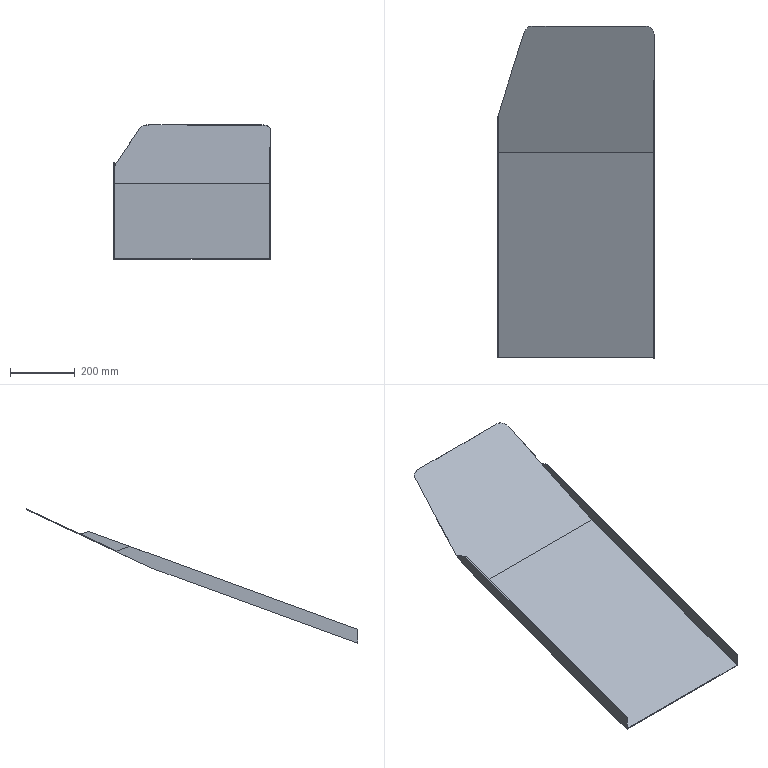Part | NX | features solid 2 | 1 solid | 17 faces | box 480.993 x 1021 x 413.434 mm | volume 1152601 mm3 | plane 14 | spline 3
STEP:
#1=CARTESIAN_POINT('',(108.81,-820.,-518.767));
#2=VERTEX_POINT('',#1);
#3=CARTESIAN_POINT('',(589.803,-820.,-518.767));
#4=VERTEX_POINT('',#3);
#5=CARTESIAN_POINT('',(1065.,-820.,-518.767));
#6=DIRECTION('',(-1.,0.,0.));
#7=VECTOR('',#6,1000.);
#8=LINE('',#5,#7);
#9=EDGE_CURVE('',#2,#4,#8,.F.);
#10=ORIENTED_EDGE('',*,*,#9,.T.);
#11=CARTESIAN_POINT('',(589.803,-820.,-476.2));
#12=VERTEX_POINT('',#11);
#13=CARTESIAN_POINT('',(589.803,-820.,-700.));
#14=DIRECTION('',(0.,0.,-1.));
#15=VECTOR('',#14,1000.);
#16=LINE('',#13,#15);
#17=EDGE_CURVE('',#12,#4,#16,.T.);
#18=ORIENTED_EDGE('',*,*,#17,.F.);
#19=CARTESIAN_POINT('',(587.803,-820.,-476.2));
#20=VERTEX_POINT('',#19);
#21=CARTESIAN_POINT('',(589.803,-820.,-476.2));
#22=DIRECTION('',(1.,0.,0.));
#23=VECTOR('',#22,1000.);
#24=LINE('',#21,#23);
#25=EDGE_CURVE('',#20,#12,#24,.T.);
#26=ORIENTED_EDGE('',*,*,#25,.F.);
#27=CARTESIAN_POINT('',(587.803,-820.,-516.639));
#28=VERTEX_POINT('',#27);
#29=CARTESIAN_POINT('',(587.803,-820.,-700.));
#30=DIRECTION('',(0.,0.,-1.));
#31=VECTOR('',#30,1000.);
#32=LINE('',#29,#31);
#33=EDGE_CURVE('',#28,#20,#32,.F.);
#34=ORIENTED_EDGE('',*,*,#33,.F.);
#35=CARTESIAN_POINT('',(110.81,-820.,-516.639));
#36=VERTEX_POINT('',#35);
#37=CARTESIAN_POINT('',(274.102,-820.,-516.639));
#38=DIRECTION('',(1.,0.,0.));
#39=VECTOR('',#38,1000.);
#40=LINE('',#37,#39);
#41=EDGE_CURVE('',#36,#28,#40,.T.);
#42=ORIENTED_EDGE('',*,*,#41,.F.);
#43=CARTESIAN_POINT('',(110.81,-820.,-476.2));
#44=VERTEX_POINT('',#43);
#45=CARTESIAN_POINT('',(110.81,-820.,-700.));
#46=DIRECTION('',(0.,0.,1.));
#47=VECTOR('',#46,1000.);
#48=LINE('',#45,#47);
#49=EDGE_CURVE('',#44,#36,#48,.F.);
#50=ORIENTED_EDGE('',*,*,#49,.F.);
#51=CARTESIAN_POINT('',(108.81,-820.,-476.2));
#52=VERTEX_POINT('',#51);
#53=CARTESIAN_POINT('',(1065.,-820.,-476.2));
#54=DIRECTION('',(1.,0.,0.));
#55=VECTOR('',#54,1000.);
#56=LINE('',#53,#55);
#57=EDGE_CURVE('',#52,#44,#56,.T.);
#58=ORIENTED_EDGE('',*,*,#57,.F.);
#59=CARTESIAN_POINT('',(108.81,-820.,-113.668));
#60=DIRECTION('',(0.,0.,1.));
#61=VECTOR('',#60,1000.);
#62=LINE('',#59,#61);
#63=EDGE_CURVE('',#2,#52,#62,.T.);
#64=ORIENTED_EDGE('',*,*,#63,.F.);
#65=EDGE_LOOP('',(#10,#18,#26,#34,#42,#50,#58,#64));
#66=FACE_BOUND('',#65,.T.);
#67=CARTESIAN_POINT('',(1065.,-820.,-700.));
#68=DIRECTION('',(0.,1.,0.));
#69=DIRECTION('',(-1.,0.,0.));
#70=AXIS2_PLACEMENT_3D('',#67,#68,#69);
#71=PLANE('',#70);
#72=ADVANCED_FACE('',(#66),#71,.F.);
#73=CARTESIAN_POINT('',(587.803,-186.962,-286.232));
#74=VERTEX_POINT('',#73);
#75=CARTESIAN_POINT('',(587.803,-188.342,-286.734));
#76=DIRECTION('',(0.,-0.9397,-0.342));
#77=VECTOR('',#76,1000.);
#78=LINE('',#75,#77);
#79=EDGE_CURVE('',#74,#28,#78,.T.);
#80=ORIENTED_EDGE('',*,*,#79,.F.);
#81=CARTESIAN_POINT('',(110.81,-186.962,-286.232));
#82=VERTEX_POINT('',#81);
#83=CARTESIAN_POINT('',(555.,-186.962,-286.232));
#84=DIRECTION('',(1.,0.,0.));
#85=VECTOR('',#84,1000.);
#86=LINE('',#83,#85);
#87=EDGE_CURVE('',#82,#74,#86,.T.);
#88=ORIENTED_EDGE('',*,*,#87,.F.);
#89=CARTESIAN_POINT('',(110.81,-188.342,-286.734));
#90=DIRECTION('',(0.,0.9397,0.342));
#91=VECTOR('',#90,1000.);
#92=LINE('',#89,#91);
#93=EDGE_CURVE('',#36,#82,#92,.T.);
#94=ORIENTED_EDGE('',*,*,#93,.F.);
#95=ORIENTED_EDGE('',*,*,#41,.T.);
#96=EDGE_LOOP('',(#80,#88,#94,#95));
#97=FACE_BOUND('',#96,.T.);
#98=CARTESIAN_POINT('',(274.102,-188.342,-286.734));
#99=DIRECTION('',(0.,0.342,-0.9397));
#100=DIRECTION('',(-1.,0.,0.));
#101=AXIS2_PLACEMENT_3D('',#98,#99,#100);
#102=PLANE('',#101);
#103=ADVANCED_FACE('',(#97),#102,.F.);
#104=ORIENTED_EDGE('',*,*,#87,.T.);
#105=CARTESIAN_POINT('',(587.803,32.739,-183.784));
#106=VERTEX_POINT('',#105);
#107=CARTESIAN_POINT('',(587.803,183.102,-113.668));
#108=DIRECTION('',(0.,0.9063,0.4226));
#109=VECTOR('',#108,1000.);
#110=LINE('',#107,#109);
#111=EDGE_CURVE('',#74,#106,#110,.T.);
#112=ORIENTED_EDGE('',*,*,#111,.T.);
#113=CARTESIAN_POINT('',(589.803,32.739,-183.784));
#114=VERTEX_POINT('',#113);
#115=CARTESIAN_POINT('',(589.803,32.739,-183.784));
#116=DIRECTION('',(1.,0.,0.));
#117=VECTOR('',#116,1000.);
#118=LINE('',#115,#117);
#119=EDGE_CURVE('',#106,#114,#118,.T.);
#120=ORIENTED_EDGE('',*,*,#119,.T.);
#121=CARTESIAN_POINT('',(589.803,33.584,-183.39));
#122=VERTEX_POINT('',#121);
#123=CARTESIAN_POINT('',(589.803,183.102,-113.668));
#124=DIRECTION('',(0.,-0.9063,-0.4226));
#125=VECTOR('',#124,1000.);
#126=LINE('',#123,#125);
#127=EDGE_CURVE('',#122,#114,#126,.T.);
#128=ORIENTED_EDGE('',*,*,#127,.F.);
#129=CARTESIAN_POINT('',(589.803,144.66,-131.594));
#130=VERTEX_POINT('',#129);
#131=CARTESIAN_POINT('',(589.803,33.584,-183.39));
#132=CARTESIAN_POINT('',(589.803,70.609,-166.125));
#133=CARTESIAN_POINT('',(589.803,107.634,-148.859));
#134=CARTESIAN_POINT('',(589.803,144.66,-131.594));
#135=B_SPLINE_CURVE_WITH_KNOTS('',3,(#131,#132,#133,#134),.UNSPECIFIED.,.F.,.F.,(4,4),(0.,1.),.UNSPECIFIED.);
#136=EDGE_CURVE('',#130,#122,#135,.F.);
#137=ORIENTED_EDGE('',*,*,#136,.F.);
#138=CARTESIAN_POINT('',(589.803,176.289,-116.845));
#139=VERTEX_POINT('',#138);
#140=CARTESIAN_POINT('',(589.803,183.102,-113.668));
#141=DIRECTION('',(0.,-0.9063,-0.4226));
#142=VECTOR('',#141,1000.);
#143=LINE('',#140,#142);
#144=EDGE_CURVE('',#139,#130,#143,.T.);
#145=ORIENTED_EDGE('',*,*,#144,.F.);
#146=CARTESIAN_POINT('',(374.989,200.501,-105.555));
#147=VERTEX_POINT('',#146);
#148=CARTESIAN_POINT('',(589.803,176.289,-116.845));
#149=CARTESIAN_POINT('',(589.689,178.459,-115.833));
#150=CARTESIAN_POINT('',(589.039,182.718,-113.847));
#151=CARTESIAN_POINT('',(586.3,188.791,-111.016));
#152=CARTESIAN_POINT('',(582.012,194.011,-108.581));
#153=CARTESIAN_POINT('',(576.33,198.,-106.721));
#154=CARTESIAN_POINT('',(569.521,200.317,-105.641));
#155=CARTESIAN_POINT('',(562.281,200.46,-105.574));
#156=CARTESIAN_POINT('',(555.087,200.407,-105.599));
#157=CARTESIAN_POINT('',(547.881,200.41,-105.597));
#158=CARTESIAN_POINT('',(540.677,200.401,-105.601));
#159=CARTESIAN_POINT('',(531.072,200.398,-105.603));
#160=CARTESIAN_POINT('',(519.066,200.397,-105.604));
#161=CARTESIAN_POINT('',(504.658,200.401,-105.602));
#162=CARTESIAN_POINT('',(485.448,200.411,-105.597));
#163=CARTESIAN_POINT('',(461.435,200.427,-105.59));
#164=CARTESIAN_POINT('',(432.62,200.445,-105.581));
#165=CARTESIAN_POINT('',(403.804,200.47,-105.569));
#166=CARTESIAN_POINT('',(384.594,200.49,-105.56));
#167=CARTESIAN_POINT('',(374.989,200.501,-105.555));
#168=B_SPLINE_CURVE_WITH_KNOTS('',3,(#148,#149,#150,#151,#152,#153,#154,#155,#156,#157,#158,#159,#160,#161,#162,#163,#164,#165,#166,#167),.UNSPECIFIED.,.F.,.F.,(4,1,1,1,1,1,1,1,1,1,1,1,1,1,1,1,1,4),(0.,0.007104,0.01421,0.02131,0.02842,0.03552,0.04263,0.04973,0.05683,0.06394,0.07104,0.08525,0.09946,0.1137,0.1421,0.1705,0.1989,0.2273),.UNSPECIFIED.);
#169=EDGE_CURVE('',#139,#147,#168,.T.);
#170=ORIENTED_EDGE('',*,*,#169,.T.);
#171=CARTESIAN_POINT('',(108.81,-77.408,-235.146));
#172=VERTEX_POINT('',#171);
#173=CARTESIAN_POINT('',(374.989,200.501,-105.555));
#174=CARTESIAN_POINT('',(364.858,200.512,-105.55));
#175=CARTESIAN_POINT('',(344.595,200.537,-105.538));
#176=CARTESIAN_POINT('',(319.267,200.578,-105.519));
#177=CARTESIAN_POINT('',(299.005,200.618,-105.5));
#178=CARTESIAN_POINT('',(283.808,200.655,-105.483));
#179=CARTESIAN_POINT('',(268.611,200.701,-105.462));
#180=CARTESIAN_POINT('',(253.415,200.754,-105.437));
#181=CARTESIAN_POINT('',(240.751,200.83,-105.402));
#182=CARTESIAN_POINT('',(230.62,200.892,-105.372));
#183=CARTESIAN_POINT('',(223.022,200.942,-105.349));
#184=CARTESIAN_POINT('',(216.683,201.04,-105.304));
#185=CARTESIAN_POINT('',(211.664,200.417,-105.594));
#186=CARTESIAN_POINT('',(206.634,199.19,-106.166));
#187=CARTESIAN_POINT('',(200.857,196.591,-107.378));
#188=CARTESIAN_POINT('',(195.037,191.859,-109.585));
#189=CARTESIAN_POINT('',(190.69,185.963,-112.334));
#190=CARTESIAN_POINT('',(187.958,179.442,-115.375));
#191=CARTESIAN_POINT('',(185.967,172.644,-118.545));
#192=CARTESIAN_POINT('',(183.9,165.886,-121.696));
#193=CARTESIAN_POINT('',(181.808,159.128,-124.848));
#194=CARTESIAN_POINT('',(179.029,150.117,-129.049));
#195=CARTESIAN_POINT('',(175.562,138.851,-134.303));
#196=CARTESIAN_POINT('',(171.409,125.33,-140.608));
#197=CARTESIAN_POINT('',(165.867,107.303,-149.014));
#198=CARTESIAN_POINT('',(158.92,84.774,-159.519));
#199=CARTESIAN_POINT('',(150.571,57.743,-172.124));
#200=CARTESIAN_POINT('',(142.222,30.712,-184.729));
#201=CARTESIAN_POINT('',(133.888,3.677,-197.335));
#202=CARTESIAN_POINT('',(122.783,-32.371,-214.145));
#203=CARTESIAN_POINT('',(114.391,-59.391,-226.745));
#204=CARTESIAN_POINT('',(108.81,-77.408,-235.146));
#205=B_SPLINE_CURVE_WITH_KNOTS('',3,(#173,#174,#175,#176,#177,#178,#179,#180,#181,#182,#183,#184,#185,#186,#187,#188,#189,#190,#191,#192,#193,#194,#195,#196,#197,#198,#199,#200,#201,#202,#203,#204),.UNSPECIFIED.,.F.,.F.,(4,1,1,1,1,1,1,1,1,1,1,1,1,1,1,1,1,1,1,1,1,1,1,1,1,1,1,1,1,4),(0.,0.03039,0.06079,0.07598,0.09118,0.1064,0.1216,0.1368,0.1444,0.152,0.1596,0.1634,0.1672,0.1748,0.1824,0.19,0.1976,0.2052,0.2128,0.2204,0.228,0.2431,0.2583,0.2735,0.3039,0.3343,0.3647,0.3951,0.4255,0.4863),.UNSPECIFIED.);
#206=EDGE_CURVE('',#147,#172,#205,.T.);
#207=ORIENTED_EDGE('',*,*,#206,.T.);
#208=CARTESIAN_POINT('',(108.81,-78.254,-235.54));
#209=VERTEX_POINT('',#208);
#210=CARTESIAN_POINT('',(108.81,183.102,-113.668));
#211=DIRECTION('',(0.,-0.9063,-0.4226));
#212=VECTOR('',#211,1000.);
#213=LINE('',#210,#212);
#214=EDGE_CURVE('',#172,#209,#213,.T.);
#215=ORIENTED_EDGE('',*,*,#214,.T.);
#216=CARTESIAN_POINT('',(110.81,-78.254,-235.54));
#217=VERTEX_POINT('',#216);
#218=CARTESIAN_POINT('',(110.81,-78.254,-235.54));
#219=DIRECTION('',(1.,0.,0.));
#220=VECTOR('',#219,1000.);
#221=LINE('',#218,#220);
#222=EDGE_CURVE('',#209,#217,#221,.T.);
#223=ORIENTED_EDGE('',*,*,#222,.T.);
#224=CARTESIAN_POINT('',(110.81,183.102,-113.668));
#225=DIRECTION('',(0.,-0.9063,-0.4226));
#226=VECTOR('',#225,1000.);
#227=LINE('',#224,#226);
#228=EDGE_CURVE('',#217,#82,#227,.T.);
#229=ORIENTED_EDGE('',*,*,#228,.T.);
#230=EDGE_LOOP('',(#104,#112,#120,#128,#137,#145,#170,#207,#215,#223,#229));
#231=FACE_BOUND('',#230,.T.);
#232=CARTESIAN_POINT('',(555.,183.102,-113.668));
#233=DIRECTION('',(0.,-0.4226,0.9063));
#234=DIRECTION('',(1.,0.,0.));
#235=AXIS2_PLACEMENT_3D('',#232,#233,#234);
#236=PLANE('',#235);
#237=ADVANCED_FACE('',(#231),#236,.T.);
#238=CARTESIAN_POINT('',(589.803,144.66,-133.801));
#239=VERTEX_POINT('',#238);
#240=CARTESIAN_POINT('',(589.803,33.584,-185.596));
#241=VERTEX_POINT('',#240);
#242=CARTESIAN_POINT('',(589.803,144.66,-133.801));
#243=CARTESIAN_POINT('',(589.803,107.634,-151.066));
#244=CARTESIAN_POINT('',(589.803,70.609,-168.331));
#245=CARTESIAN_POINT('',(589.803,33.584,-185.596));
#246=B_SPLINE_CURVE_WITH_KNOTS('',3,(#242,#243,#244,#245),.UNSPECIFIED.,.F.,.F.,(4,4),(0.,1.),.UNSPECIFIED.);
#247=EDGE_CURVE('',#239,#241,#246,.T.);
#248=ORIENTED_EDGE('',*,*,#247,.T.);
#249=CARTESIAN_POINT('',(589.803,-186.196,-288.081));
#250=VERTEX_POINT('',#249);
#251=CARTESIAN_POINT('',(589.803,183.947,-115.481));
#252=DIRECTION('',(0.,-0.9063,-0.4226));
#253=VECTOR('',#252,1000.);
#254=LINE('',#251,#253);
#255=EDGE_CURVE('',#250,#241,#254,.F.);
#256=ORIENTED_EDGE('',*,*,#255,.F.);
#257=CARTESIAN_POINT('',(108.81,-186.196,-288.081));
#258=VERTEX_POINT('',#257);
#259=CARTESIAN_POINT('',(274.102,-186.196,-288.081));
#260=DIRECTION('',(-1.,0.,0.));
#261=VECTOR('',#260,1000.);
#262=LINE('',#259,#261);
#263=EDGE_CURVE('',#258,#250,#262,.F.);
#264=ORIENTED_EDGE('',*,*,#263,.F.);
#265=CARTESIAN_POINT('',(108.81,-77.408,-237.353));
#266=VERTEX_POINT('',#265);
#267=CARTESIAN_POINT('',(108.81,183.947,-115.481));
#268=DIRECTION('',(0.,-0.9063,-0.4226));
#269=VECTOR('',#268,1000.);
#270=LINE('',#267,#269);
#271=EDGE_CURVE('',#258,#266,#270,.F.);
#272=ORIENTED_EDGE('',*,*,#271,.T.);
#273=CARTESIAN_POINT('',(374.989,200.501,-107.762));
#274=VERTEX_POINT('',#273);
#275=CARTESIAN_POINT('',(374.989,200.501,-107.762));
#276=CARTESIAN_POINT('',(364.858,200.512,-107.756));
#277=CARTESIAN_POINT('',(344.595,200.537,-107.745));
#278=CARTESIAN_POINT('',(319.267,200.578,-107.726));
#279=CARTESIAN_POINT('',(299.005,200.618,-107.707));
#280=CARTESIAN_POINT('',(283.808,200.655,-107.69));
#281=CARTESIAN_POINT('',(268.611,200.701,-107.669));
#282=CARTESIAN_POINT('',(253.415,200.754,-107.644));
#283=CARTESIAN_POINT('',(240.751,200.83,-107.608));
#284=CARTESIAN_POINT('',(230.62,200.892,-107.579));
#285=CARTESIAN_POINT('',(223.022,200.942,-107.556));
#286=CARTESIAN_POINT('',(216.683,201.04,-107.51));
#287=CARTESIAN_POINT('',(211.664,200.417,-107.801));
#288=CARTESIAN_POINT('',(206.634,199.19,-108.373));
#289=CARTESIAN_POINT('',(200.857,196.591,-109.585));
#290=CARTESIAN_POINT('',(195.037,191.859,-111.792));
#291=CARTESIAN_POINT('',(190.69,185.963,-114.541));
#292=CARTESIAN_POINT('',(187.958,179.442,-117.582));
#293=CARTESIAN_POINT('',(185.967,172.644,-120.752));
#294=CARTESIAN_POINT('',(183.9,165.886,-123.903));
#295=CARTESIAN_POINT('',(181.808,159.128,-127.054));
#296=CARTESIAN_POINT('',(179.029,150.117,-131.256));
#297=CARTESIAN_POINT('',(175.562,138.851,-136.51));
#298=CARTESIAN_POINT('',(171.409,125.33,-142.815));
#299=CARTESIAN_POINT('',(165.867,107.303,-151.221));
#300=CARTESIAN_POINT('',(158.92,84.774,-161.726));
#301=CARTESIAN_POINT('',(150.571,57.743,-174.331));
#302=CARTESIAN_POINT('',(142.222,30.712,-186.936));
#303=CARTESIAN_POINT('',(133.888,3.677,-199.542));
#304=CARTESIAN_POINT('',(122.783,-32.371,-216.352));
#305=CARTESIAN_POINT('',(114.391,-59.391,-228.951));
#306=CARTESIAN_POINT('',(108.81,-77.408,-237.353));
#307=B_SPLINE_CURVE_WITH_KNOTS('',3,(#275,#276,#277,#278,#279,#280,#281,#282,#283,#284,#285,#286,#287,#288,#289,#290,#291,#292,#293,#294,#295,#296,#297,#298,#299,#300,#301,#302,#303,#304,#305,#306),.UNSPECIFIED.,.F.,.F.,(4,1,1,1,1,1,1,1,1,1,1,1,1,1,1,1,1,1,1,1,1,1,1,1,1,1,1,1,1,4),(0.,0.03039,0.06079,0.07598,0.09118,0.1064,0.1216,0.1368,0.1444,0.152,0.1596,0.1634,0.1672,0.1748,0.1824,0.19,0.1976,0.2052,0.2128,0.2204,0.228,0.2431,0.2583,0.2735,0.3039,0.3343,0.3647,0.3951,0.4255,0.4863),.UNSPECIFIED.);
#308=EDGE_CURVE('',#274,#266,#307,.T.);
#309=ORIENTED_EDGE('',*,*,#308,.F.);
#310=CARTESIAN_POINT('',(589.803,176.289,-119.052));
#311=VERTEX_POINT('',#310);
#312=CARTESIAN_POINT('',(589.803,176.289,-119.052));
#313=CARTESIAN_POINT('',(589.689,178.459,-118.04));
#314=CARTESIAN_POINT('',(589.039,182.718,-116.054));
#315=CARTESIAN_POINT('',(586.3,188.791,-113.222));
#316=CARTESIAN_POINT('',(582.012,194.011,-110.788));
#317=CARTESIAN_POINT('',(576.33,198.,-108.928));
#318=CARTESIAN_POINT('',(569.521,200.317,-107.848));
#319=CARTESIAN_POINT('',(562.281,200.46,-107.781));
#320=CARTESIAN_POINT('',(555.087,200.407,-107.805));
#321=CARTESIAN_POINT('',(547.881,200.41,-107.804));
#322=CARTESIAN_POINT('',(540.677,200.401,-107.808));
#323=CARTESIAN_POINT('',(531.072,200.398,-107.81));
#324=CARTESIAN_POINT('',(519.066,200.397,-107.81));
#325=CARTESIAN_POINT('',(504.658,200.401,-107.808));
#326=CARTESIAN_POINT('',(485.448,200.411,-107.804));
#327=CARTESIAN_POINT('',(461.435,200.427,-107.796));
#328=CARTESIAN_POINT('',(432.62,200.445,-107.788));
#329=CARTESIAN_POINT('',(403.804,200.47,-107.776));
#330=CARTESIAN_POINT('',(384.594,200.49,-107.767));
#331=CARTESIAN_POINT('',(374.989,200.501,-107.762));
#332=B_SPLINE_CURVE_WITH_KNOTS('',3,(#312,#313,#314,#315,#316,#317,#318,#319,#320,#321,#322,#323,#324,#325,#326,#327,#328,#329,#330,#331),.UNSPECIFIED.,.F.,.F.,(4,1,1,1,1,1,1,1,1,1,1,1,1,1,1,1,1,4),(0.,0.007104,0.01421,0.02131,0.02842,0.03552,0.04263,0.04973,0.05683,0.06394,0.07104,0.08525,0.09946,0.1137,0.1421,0.1705,0.1989,0.2273),.UNSPECIFIED.);
#333=EDGE_CURVE('',#311,#274,#332,.T.);
#334=ORIENTED_EDGE('',*,*,#333,.F.);
#335=CARTESIAN_POINT('',(589.803,183.947,-115.481));
#336=DIRECTION('',(0.,-0.9063,-0.4226));
#337=VECTOR('',#336,1000.);
#338=LINE('',#335,#337);
#339=EDGE_CURVE('',#311,#239,#338,.T.);
#340=ORIENTED_EDGE('',*,*,#339,.T.);
#341=EDGE_LOOP('',(#248,#256,#264,#272,#309,#334,#340));
#342=FACE_BOUND('',#341,.T.);
#343=CARTESIAN_POINT('',(555.,183.947,-115.481));
#344=DIRECTION('',(0.,-0.4226,0.9063));
#345=DIRECTION('',(1.,0.,0.));
#346=AXIS2_PLACEMENT_3D('',#343,#344,#345);
#347=PLANE('',#346);
#348=ADVANCED_FACE('',(#342),#347,.F.);
#349=CARTESIAN_POINT('',(589.803,-187.658,-288.613));
#350=DIRECTION('',(0.,-0.9397,-0.342));
#351=VECTOR('',#350,1000.);
#352=LINE('',#349,#351);
#353=EDGE_CURVE('',#250,#4,#352,.T.);
#354=ORIENTED_EDGE('',*,*,#353,.T.);
#355=ORIENTED_EDGE('',*,*,#9,.F.);
#356=CARTESIAN_POINT('',(108.81,-187.658,-288.613));
#357=DIRECTION('',(0.,-0.9397,-0.342));
#358=VECTOR('',#357,1000.);
#359=LINE('',#356,#358);
#360=EDGE_CURVE('',#258,#2,#359,.T.);
#361=ORIENTED_EDGE('',*,*,#360,.F.);
#362=ORIENTED_EDGE('',*,*,#263,.T.);
#363=EDGE_LOOP('',(#354,#355,#361,#362));
#364=FACE_BOUND('',#363,.T.);
#365=CARTESIAN_POINT('',(274.102,-187.658,-288.613));
#366=DIRECTION('',(0.,0.342,-0.9397));
#367=DIRECTION('',(-1.,0.,0.));
#368=AXIS2_PLACEMENT_3D('',#365,#366,#367);
#369=PLANE('',#368);
#370=ADVANCED_FACE('',(#364),#369,.T.);
#371=ORIENTED_EDGE('',*,*,#360,.T.);
#372=ORIENTED_EDGE('',*,*,#63,.T.);
#373=CARTESIAN_POINT('',(108.81,-118.523,-220.883));
#374=VERTEX_POINT('',#373);
#375=CARTESIAN_POINT('',(108.81,182.276,-111.401));
#376=DIRECTION('',(0.,-0.9397,-0.342));
#377=VECTOR('',#376,1000.);
#378=LINE('',#375,#377);
#379=EDGE_CURVE('',#374,#52,#378,.T.);
#380=ORIENTED_EDGE('',*,*,#379,.F.);
#381=CARTESIAN_POINT('',(108.81,-78.254,-235.54));
#382=DIRECTION('',(0.,-0.9397,0.342));
#383=VECTOR('',#382,1000.);
#384=LINE('',#381,#383);
#385=EDGE_CURVE('',#374,#209,#384,.F.);
#386=ORIENTED_EDGE('',*,*,#385,.T.);
#387=ORIENTED_EDGE('',*,*,#214,.F.);
#388=CARTESIAN_POINT('',(108.81,-77.408,-1000.));
#389=DIRECTION('',(0.,0.,1.));
#390=VECTOR('',#389,1000.);
#391=LINE('',#388,#390);
#392=EDGE_CURVE('',#266,#172,#391,.T.);
#393=ORIENTED_EDGE('',*,*,#392,.F.);
#394=ORIENTED_EDGE('',*,*,#271,.F.);
#395=EDGE_LOOP('',(#371,#372,#380,#386,#387,#393,#394));
#396=FACE_BOUND('',#395,.T.);
#397=CARTESIAN_POINT('',(108.81,183.102,-113.668));
#398=DIRECTION('',(1.,0.,0.));
#399=DIRECTION('',(0.,0.,-1.));
#400=AXIS2_PLACEMENT_3D('',#397,#398,#399);
#401=PLANE('',#400);
#402=ADVANCED_FACE('',(#396),#401,.F.);
#403=ORIENTED_EDGE('',*,*,#17,.T.);
#404=ORIENTED_EDGE('',*,*,#353,.F.);
#405=ORIENTED_EDGE('',*,*,#255,.T.);
#406=CARTESIAN_POINT('',(589.803,33.584,-1000.));
#407=DIRECTION('',(0.,0.,1.));
#408=VECTOR('',#407,1000.);
#409=LINE('',#406,#408);
#410=EDGE_CURVE('',#241,#122,#409,.T.);
#411=ORIENTED_EDGE('',*,*,#410,.T.);
#412=ORIENTED_EDGE('',*,*,#127,.T.);
#413=CARTESIAN_POINT('',(589.803,8.073,-174.806));
#414=VERTEX_POINT('',#413);
#415=CARTESIAN_POINT('',(589.803,8.818,-175.077));
#416=DIRECTION('',(0.,-0.9397,0.342));
#417=VECTOR('',#416,1000.);
#418=LINE('',#415,#417);
#419=EDGE_CURVE('',#114,#414,#418,.T.);
#420=ORIENTED_EDGE('',*,*,#419,.T.);
#421=CARTESIAN_POINT('',(589.803,-199.877,-250.494));
#422=DIRECTION('',(0.,-0.9397,-0.342));
#423=VECTOR('',#422,1000.);
#424=LINE('',#421,#423);
#425=EDGE_CURVE('',#414,#12,#424,.T.);
#426=ORIENTED_EDGE('',*,*,#425,.T.);
#427=EDGE_LOOP('',(#403,#404,#405,#411,#412,#420,#426));
#428=FACE_BOUND('',#427,.T.);
#429=CARTESIAN_POINT('',(589.803,183.102,-113.668));
#430=DIRECTION('',(1.,0.,0.));
#431=DIRECTION('',(0.,0.,-1.));
#432=AXIS2_PLACEMENT_3D('',#429,#430,#431);
#433=PLANE('',#432);
#434=ADVANCED_FACE('',(#428),#433,.T.);
#435=ORIENTED_EDGE('',*,*,#206,.F.);
#436=CARTESIAN_POINT('',(374.989,200.501,-1000.));
#437=DIRECTION('',(0.,0.,1.));
#438=VECTOR('',#437,1000.);
#439=LINE('',#436,#438);
#440=EDGE_CURVE('',#274,#147,#439,.T.);
#441=ORIENTED_EDGE('',*,*,#440,.F.);
#442=ORIENTED_EDGE('',*,*,#308,.T.);
#443=ORIENTED_EDGE('',*,*,#392,.T.);
#444=EDGE_LOOP('',(#435,#441,#442,#443));
#445=FACE_BOUND('',#444,.T.);
#446=CARTESIAN_POINT('',(374.989,200.501,-238.148));
#447=CARTESIAN_POINT('',(374.989,200.501,-104.13));
#448=CARTESIAN_POINT('',(365.187,200.512,-238.148));
#449=CARTESIAN_POINT('',(365.187,200.512,-104.13));
#450=CARTESIAN_POINT('',(345.583,200.536,-238.148));
#451=CARTESIAN_POINT('',(345.583,200.536,-104.13));
#452=CARTESIAN_POINT('',(316.178,200.583,-238.148));
#453=CARTESIAN_POINT('',(316.178,200.583,-104.13));
#454=CARTESIAN_POINT('',(291.673,200.633,-238.148));
#455=CARTESIAN_POINT('',(291.673,200.633,-104.13));
#456=CARTESIAN_POINT('',(272.069,200.689,-238.148));
#457=CARTESIAN_POINT('',(272.069,200.689,-104.13));
#458=CARTESIAN_POINT('',(257.367,200.742,-238.148));
#459=CARTESIAN_POINT('',(257.367,200.742,-104.13));
#460=CARTESIAN_POINT('',(245.114,200.793,-238.148));
#461=CARTESIAN_POINT('',(245.114,200.793,-104.13));
#462=CARTESIAN_POINT('',(235.313,200.874,-238.148));
#463=CARTESIAN_POINT('',(235.313,200.874,-104.13));
#464=CARTESIAN_POINT('',(227.961,200.88,-238.148));
#465=CARTESIAN_POINT('',(227.961,200.88,-104.13));
#466=CARTESIAN_POINT('',(220.611,201.039,-238.148));
#467=CARTESIAN_POINT('',(220.611,201.039,-104.13));
#468=CARTESIAN_POINT('',(213.256,200.864,-238.148));
#469=CARTESIAN_POINT('',(213.256,200.864,-104.13));
#470=CARTESIAN_POINT('',(206.093,199.101,-238.148));
#471=CARTESIAN_POINT('',(206.093,199.101,-104.13));
#472=CARTESIAN_POINT('',(199.581,195.744,-238.148));
#473=CARTESIAN_POINT('',(199.581,195.744,-104.13));
#474=CARTESIAN_POINT('',(194.084,190.795,-238.148));
#475=CARTESIAN_POINT('',(194.084,190.795,-104.13));
#476=CARTESIAN_POINT('',(189.965,184.643,-238.148));
#477=CARTESIAN_POINT('',(189.965,184.643,-104.13));
#478=CARTESIAN_POINT('',(187.476,177.842,-238.148));
#479=CARTESIAN_POINT('',(187.476,177.842,-104.13));
#480=CARTESIAN_POINT('',(185.452,170.916,-238.148));
#481=CARTESIAN_POINT('',(185.452,170.916,-104.13));
#482=CARTESIAN_POINT('',(183.32,164.017,-238.148));
#483=CARTESIAN_POINT('',(183.32,164.017,-104.13));
#484=CARTESIAN_POINT('',(180.478,154.822,-238.148));
#485=CARTESIAN_POINT('',(180.478,154.822,-104.13));
#486=CARTESIAN_POINT('',(176.937,143.323,-238.148));
#487=CARTESIAN_POINT('',(176.937,143.323,-104.13));
#488=CARTESIAN_POINT('',(172.697,129.522,-238.148));
#489=CARTESIAN_POINT('',(172.697,129.522,-104.13));
#490=CARTESIAN_POINT('',(167.043,111.12,-238.148));
#491=CARTESIAN_POINT('',(167.043,111.12,-104.13));
#492=CARTESIAN_POINT('',(159.955,88.125,-238.148));
#493=CARTESIAN_POINT('',(159.955,88.125,-104.13));
#494=CARTESIAN_POINT('',(151.434,60.535,-238.148));
#495=CARTESIAN_POINT('',(151.434,60.535,-104.13));
#496=CARTESIAN_POINT('',(142.911,32.946,-238.148));
#497=CARTESIAN_POINT('',(142.911,32.946,-104.13));
#498=CARTESIAN_POINT('',(134.404,5.352,-238.148));
#499=CARTESIAN_POINT('',(134.404,5.352,-104.13));
#500=CARTESIAN_POINT('',(123.07,-31.443,-238.148));
#501=CARTESIAN_POINT('',(123.07,-31.443,-104.13));
#502=CARTESIAN_POINT('',(114.506,-59.02,-238.148));
#503=CARTESIAN_POINT('',(114.506,-59.02,-104.13));
#504=CARTESIAN_POINT('',(108.81,-77.408,-238.148));
#505=CARTESIAN_POINT('',(108.81,-77.408,-104.13));
#506=B_SPLINE_SURFACE_WITH_KNOTS('',3,1,((#446,#447),(#448,#449),(#450,#451),(#452,#453),(#454,#455),(#456,#457),(#458,#459),(#460,#461),(#462,#463),(#464,#465),(#466,#467),(#468,#469),(#470,#471),(#472,#473),(#474,#475),(#476,#477),(#478,#479),(#480,#481),(#482,#483),(#484,#485),(#486,#487),(#488,#489),(#490,#491),(#492,#493),(#494,#495),(#496,#497),(#498,#499),(#500,#501),(#502,#503),(#504,#505)),.SURF_OF_LINEAR_EXTRUSION.,.F.,.F.,.F.,(4,1,1,1,1,1,1,1,1,1,1,1,1,1,1,1,1,1,1,1,1,1,1,1,1,1,1,4),(2,2),(0.,0.03647,0.07294,0.1094,0.1276,0.1459,0.1641,0.1732,0.1823,0.1915,0.2006,0.2097,0.2188,0.2279,0.237,0.2462,0.2553,0.2644,0.2735,0.2917,0.31,0.3282,0.3647,0.4011,0.4376,0.4741,0.5105,0.5835),(0.,1.),.UNSPECIFIED.);
#507=ADVANCED_FACE('',(#445),#506,.T.);
#508=ORIENTED_EDGE('',*,*,#169,.F.);
#509=CARTESIAN_POINT('',(589.803,176.289,-1000.));
#510=DIRECTION('',(0.,0.,1.));
#511=VECTOR('',#510,1000.);
#512=LINE('',#509,#511);
#513=EDGE_CURVE('',#311,#139,#512,.T.);
#514=ORIENTED_EDGE('',*,*,#513,.F.);
#515=ORIENTED_EDGE('',*,*,#333,.T.);
#516=ORIENTED_EDGE('',*,*,#440,.T.);
#517=EDGE_LOOP('',(#508,#514,#515,#516));
#518=FACE_BOUND('',#517,.T.);
#519=CARTESIAN_POINT('',(589.803,176.289,-119.135));
#520=CARTESIAN_POINT('',(589.803,176.289,-105.202));
#521=CARTESIAN_POINT('',(589.678,178.665,-119.135));
#522=CARTESIAN_POINT('',(589.678,178.665,-105.202));
#523=CARTESIAN_POINT('',(588.891,183.392,-119.135));
#524=CARTESIAN_POINT('',(588.891,183.392,-105.202));
#525=CARTESIAN_POINT('',(585.663,189.846,-119.135));
#526=CARTESIAN_POINT('',(585.663,189.846,-105.202));
#527=CARTESIAN_POINT('',(580.768,195.13,-119.135));
#528=CARTESIAN_POINT('',(580.768,195.13,-105.202));
#529=CARTESIAN_POINT('',(574.583,198.83,-119.135));
#530=CARTESIAN_POINT('',(574.583,198.83,-105.202));
#531=CARTESIAN_POINT('',(567.576,200.534,-119.135));
#532=CARTESIAN_POINT('',(567.576,200.534,-105.202));
#533=CARTESIAN_POINT('',(560.418,200.398,-119.135));
#534=CARTESIAN_POINT('',(560.418,200.398,-105.202));
#535=CARTESIAN_POINT('',(553.293,200.42,-119.135));
#536=CARTESIAN_POINT('',(553.293,200.42,-105.202));
#537=CARTESIAN_POINT('',(543.781,200.4,-119.135));
#538=CARTESIAN_POINT('',(543.781,200.4,-105.202));
#539=CARTESIAN_POINT('',(531.896,200.399,-119.135));
#540=CARTESIAN_POINT('',(531.896,200.399,-105.202));
#541=CARTESIAN_POINT('',(517.631,200.397,-119.135));
#542=CARTESIAN_POINT('',(517.631,200.397,-105.202));
#543=CARTESIAN_POINT('',(503.367,200.401,-119.135));
#544=CARTESIAN_POINT('',(503.367,200.401,-105.202));
#545=CARTESIAN_POINT('',(484.348,200.411,-119.135));
#546=CARTESIAN_POINT('',(484.348,200.411,-105.202));
#547=CARTESIAN_POINT('',(460.574,200.427,-119.135));
#548=CARTESIAN_POINT('',(460.574,200.427,-105.202));
#549=CARTESIAN_POINT('',(432.046,200.446,-119.135));
#550=CARTESIAN_POINT('',(432.046,200.446,-105.202));
#551=CARTESIAN_POINT('',(403.518,200.47,-119.135));
#552=CARTESIAN_POINT('',(403.518,200.47,-105.202));
#553=CARTESIAN_POINT('',(384.499,200.49,-119.135));
#554=CARTESIAN_POINT('',(384.499,200.49,-105.202));
#555=CARTESIAN_POINT('',(374.989,200.501,-119.135));
#556=CARTESIAN_POINT('',(374.989,200.501,-105.202));
#557=B_SPLINE_SURFACE_WITH_KNOTS('',3,1,((#519,#520),(#521,#522),(#523,#524),(#525,#526),(#527,#528),(#529,#530),(#531,#532),(#533,#534),(#535,#536),(#537,#538),(#539,#540),(#541,#542),(#543,#544),(#545,#546),(#547,#548),(#549,#550),(#551,#552),(#553,#554),(#555,#556)),.SURF_OF_LINEAR_EXTRUSION.,.F.,.F.,.F.,(4,1,1,1,1,1,1,1,1,1,1,1,1,1,1,1,4),(2,2),(0.6964,0.7059,0.7154,0.7249,0.7344,0.7439,0.7533,0.7628,0.7723,0.7913,0.8103,0.8292,0.8482,0.8862,0.9241,0.9621,1.),(0.,1.),.UNSPECIFIED.);
#558=ADVANCED_FACE('',(#518),#557,.T.);
#559=ORIENTED_EDGE('',*,*,#144,.T.);
#560=CARTESIAN_POINT('',(589.803,144.66,-1000.));
#561=DIRECTION('',(0.,0.,1.));
#562=VECTOR('',#561,1000.);
#563=LINE('',#560,#562);
#564=EDGE_CURVE('',#130,#239,#563,.F.);
#565=ORIENTED_EDGE('',*,*,#564,.T.);
#566=ORIENTED_EDGE('',*,*,#339,.F.);
#567=ORIENTED_EDGE('',*,*,#513,.T.);
#568=EDGE_LOOP('',(#559,#565,#566,#567));
#569=FACE_BOUND('',#568,.T.);
#570=CARTESIAN_POINT('',(589.803,183.102,-113.668));
#571=DIRECTION('',(1.,0.,0.));
#572=DIRECTION('',(0.,0.,-1.));
#573=AXIS2_PLACEMENT_3D('',#570,#571,#572);
#574=PLANE('',#573);
#575=ADVANCED_FACE('',(#569),#574,.T.);
#576=ORIENTED_EDGE('',*,*,#564,.F.);
#577=ORIENTED_EDGE('',*,*,#136,.T.);
#578=ORIENTED_EDGE('',*,*,#410,.F.);
#579=ORIENTED_EDGE('',*,*,#247,.F.);
#580=EDGE_LOOP('',(#576,#577,#578,#579));
#581=FACE_BOUND('',#580,.T.);
#582=CARTESIAN_POINT('',(589.803,33.584,-185.92));
#583=CARTESIAN_POINT('',(589.803,33.584,-131.27));
#584=CARTESIAN_POINT('',(589.796,70.609,-185.92));
#585=CARTESIAN_POINT('',(589.796,70.609,-131.27));
#586=CARTESIAN_POINT('',(589.779,107.634,-185.92));
#587=CARTESIAN_POINT('',(589.779,107.634,-131.27));
#588=CARTESIAN_POINT('',(589.803,144.66,-185.92));
#589=CARTESIAN_POINT('',(589.803,144.66,-131.27));
#590=B_SPLINE_SURFACE_WITH_KNOTS('',3,1,((#582,#583),(#584,#585),(#586,#587),(#588,#589)),.SURF_OF_LINEAR_EXTRUSION.,.F.,.F.,.F.,(4,4),(2,2),(0.5066,0.6544),(0.,1.),.PIECEWISE_BEZIER_KNOTS.);
#591=ADVANCED_FACE('',(#581),#590,.T.);
#592=ORIENTED_EDGE('',*,*,#49,.T.);
#593=ORIENTED_EDGE('',*,*,#93,.T.);
#594=ORIENTED_EDGE('',*,*,#228,.F.);
#595=CARTESIAN_POINT('',(110.81,-118.523,-220.883));
#596=VERTEX_POINT('',#595);
#597=CARTESIAN_POINT('',(110.81,-78.254,-235.54));
#598=DIRECTION('',(0.,-0.9397,0.342));
#599=VECTOR('',#598,1000.);
#600=LINE('',#597,#599);
#601=EDGE_CURVE('',#217,#596,#600,.T.);
#602=ORIENTED_EDGE('',*,*,#601,.T.);
#603=CARTESIAN_POINT('',(110.81,-199.877,-250.494));
#604=DIRECTION('',(0.,-0.9397,-0.342));
#605=VECTOR('',#604,1000.);
#606=LINE('',#603,#605);
#607=EDGE_CURVE('',#596,#44,#606,.T.);
#608=ORIENTED_EDGE('',*,*,#607,.T.);
#609=EDGE_LOOP('',(#592,#593,#594,#602,#608));
#610=FACE_BOUND('',#609,.T.);
#611=CARTESIAN_POINT('',(110.81,-186.196,-288.081));
#612=DIRECTION('',(-1.,0.,0.));
#613=DIRECTION('',(0.,-0.9397,-0.342));
#614=AXIS2_PLACEMENT_3D('',#611,#612,#613);
#615=PLANE('',#614);
#616=ADVANCED_FACE('',(#610),#615,.F.);
#617=ORIENTED_EDGE('',*,*,#379,.T.);
#618=ORIENTED_EDGE('',*,*,#57,.T.);
#619=ORIENTED_EDGE('',*,*,#607,.F.);
#620=CARTESIAN_POINT('',(108.81,-118.523,-220.883));
#621=DIRECTION('',(-1.,0.,0.));
#622=VECTOR('',#621,1000.);
#623=LINE('',#620,#622);
#624=EDGE_CURVE('',#374,#596,#623,.F.);
#625=ORIENTED_EDGE('',*,*,#624,.F.);
#626=EDGE_LOOP('',(#617,#618,#619,#625));
#627=FACE_BOUND('',#626,.T.);
#628=CARTESIAN_POINT('',(108.81,-199.877,-250.494));
#629=DIRECTION('',(0.,-0.342,0.9397));
#630=DIRECTION('',(0.,-0.9397,-0.342));
#631=AXIS2_PLACEMENT_3D('',#628,#629,#630);
#632=PLANE('',#631);
#633=ADVANCED_FACE('',(#627),#632,.T.);
#634=ORIENTED_EDGE('',*,*,#385,.F.);
#635=ORIENTED_EDGE('',*,*,#624,.T.);
#636=ORIENTED_EDGE('',*,*,#601,.F.);
#637=ORIENTED_EDGE('',*,*,#222,.F.);
#638=EDGE_LOOP('',(#634,#635,#636,#637));
#639=FACE_BOUND('',#638,.T.);
#640=CARTESIAN_POINT('',(108.81,-78.254,-235.54));
#641=DIRECTION('',(0.,0.342,0.9397));
#642=DIRECTION('',(0.,-0.9397,0.342));
#643=AXIS2_PLACEMENT_3D('',#640,#641,#642);
#644=PLANE('',#643);
#645=ADVANCED_FACE('',(#639),#644,.T.);
#646=ORIENTED_EDGE('',*,*,#79,.T.);
#647=ORIENTED_EDGE('',*,*,#33,.T.);
#648=CARTESIAN_POINT('',(587.803,8.073,-174.806));
#649=VERTEX_POINT('',#648);
#650=CARTESIAN_POINT('',(587.803,-199.877,-250.494));
#651=DIRECTION('',(0.,-0.9397,-0.342));
#652=VECTOR('',#651,1000.);
#653=LINE('',#650,#652);
#654=EDGE_CURVE('',#649,#20,#653,.T.);
#655=ORIENTED_EDGE('',*,*,#654,.F.);
#656=CARTESIAN_POINT('',(587.803,8.818,-175.077));
#657=DIRECTION('',(0.,-0.9397,0.342));
#658=VECTOR('',#657,1000.);
#659=LINE('',#656,#658);
#660=EDGE_CURVE('',#649,#106,#659,.F.);
#661=ORIENTED_EDGE('',*,*,#660,.T.);
#662=ORIENTED_EDGE('',*,*,#111,.F.);
#663=EDGE_LOOP('',(#646,#647,#655,#661,#662));
#664=FACE_BOUND('',#663,.T.);
#665=CARTESIAN_POINT('',(587.803,33.584,-185.596));
#666=DIRECTION('',(1.,0.,0.));
#667=DIRECTION('',(0.,-0.9063,-0.4226));
#668=AXIS2_PLACEMENT_3D('',#665,#666,#667);
#669=PLANE('',#668);
#670=ADVANCED_FACE('',(#664),#669,.F.);
#671=ORIENTED_EDGE('',*,*,#654,.T.);
#672=ORIENTED_EDGE('',*,*,#25,.T.);
#673=ORIENTED_EDGE('',*,*,#425,.F.);
#674=CARTESIAN_POINT('',(589.803,8.073,-174.806));
#675=DIRECTION('',(-1.,0.,0.));
#676=VECTOR('',#675,1000.);
#677=LINE('',#674,#676);
#678=EDGE_CURVE('',#649,#414,#677,.F.);
#679=ORIENTED_EDGE('',*,*,#678,.F.);
#680=EDGE_LOOP('',(#671,#672,#673,#679));
#681=FACE_BOUND('',#680,.T.);
#682=CARTESIAN_POINT('',(589.803,-199.877,-250.494));
#683=DIRECTION('',(0.,0.342,-0.9397));
#684=DIRECTION('',(0.,0.9397,0.342));
#685=AXIS2_PLACEMENT_3D('',#682,#683,#684);
#686=PLANE('',#685);
#687=ADVANCED_FACE('',(#681),#686,.F.);
#688=ORIENTED_EDGE('',*,*,#419,.F.);
#689=ORIENTED_EDGE('',*,*,#119,.F.);
#690=ORIENTED_EDGE('',*,*,#660,.F.);
#691=ORIENTED_EDGE('',*,*,#678,.T.);
#692=EDGE_LOOP('',(#688,#689,#690,#691));
#693=FACE_BOUND('',#692,.T.);
#694=CARTESIAN_POINT('',(589.803,8.818,-175.077));
#695=DIRECTION('',(0.,-0.342,-0.9397));
#696=DIRECTION('',(0.,0.9397,-0.342));
#697=AXIS2_PLACEMENT_3D('',#694,#695,#696);
#698=PLANE('',#697);
#699=ADVANCED_FACE('',(#693),#698,.F.);
#700=CLOSED_SHELL('',(#72,#103,#237,#348,#370,#402,#434,#507,#558,#575,#591,#616,#633,#645,#670,#687,#699));
#701=MANIFOLD_SOLID_BREP('',#700);
#702=(LENGTH_UNIT()NAMED_UNIT(*)SI_UNIT(.MILLI.,.METRE.));
#703=UNCERTAINTY_MEASURE_WITH_UNIT(LENGTH_MEASURE(0.0508),#702,'','');
#704=(NAMED_UNIT(*)PLANE_ANGLE_UNIT()SI_UNIT($,.RADIAN.));
#705=(NAMED_UNIT(*)SI_UNIT($,.STERADIAN.)SOLID_ANGLE_UNIT());
#706=(GEOMETRIC_REPRESENTATION_CONTEXT(3)GLOBAL_UNCERTAINTY_ASSIGNED_CONTEXT((#703))GLOBAL_UNIT_ASSIGNED_CONTEXT((#702,#704,#705))REPRESENTATION_CONTEXT('',''));
#707=ADVANCED_BREP_SHAPE_REPRESENTATION('',(#701),#706);